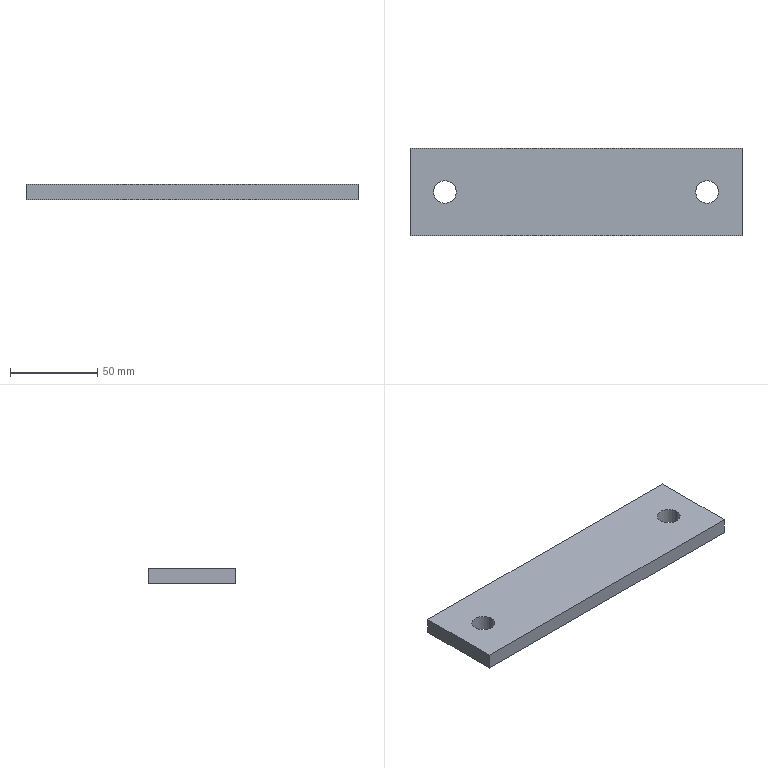Part | STEP file | DCV-000-026 | 1 solid | 10 faces | box 190 x 50 x 9 mm | volume 83111 mm3 | plane 6 | cylinder 4 | commonest cylinder face diameters 13 x4
STEP:
#1=CARTESIAN_POINT('',(0.,0.,0.));
#2=DIRECTION('',(0.,0.,1.));
#3=DIRECTION('',(1.,0.,0.));
#4=AXIS2_PLACEMENT_3D('',#1,#2,#3);
#5=CARTESIAN_POINT('',(81.5,0.,0.));
#6=VERTEX_POINT('',#5);
#7=CARTESIAN_POINT('',(81.5,0.,9.));
#8=VERTEX_POINT('',#7);
#9=CARTESIAN_POINT('',(81.5,0.,-187.675));
#10=DIRECTION('',(0.,0.,1.));
#11=VECTOR('',#10,1.);
#12=LINE('',#9,#11);
#13=CARTESIAN_POINT('',(75.,0.,-187.675));
#14=DIRECTION('',(0.,0.,1.));
#15=DIRECTION('',(1.,0.,0.));
#16=AXIS2_PLACEMENT_3D('',#13,#14,#15);
#17=CYLINDRICAL_SURFACE('',#16,6.5);
#18=CARTESIAN_POINT('',(6.283,0.));
#19=DIRECTION('',(0.,1.));
#20=VECTOR('',#19,1.);
#21=LINE('',#18,#20);
#22=(GEOMETRIC_REPRESENTATION_CONTEXT(2)PARAMETRIC_REPRESENTATION_CONTEXT()REPRESENTATION_CONTEXT('',''));
#23=DEFINITIONAL_REPRESENTATION('',(#21),#22);
#24=PCURVE('',#17,#23);
#25=CARTESIAN_POINT('',(75.,0.,-187.675));
#26=DIRECTION('',(0.,0.,1.));
#27=DIRECTION('',(1.,0.,0.));
#28=AXIS2_PLACEMENT_3D('',#25,#26,#27);
#29=CYLINDRICAL_SURFACE('',#28,6.5);
#30=CARTESIAN_POINT('',(0.,0.));
#31=DIRECTION('',(0.,1.));
#32=VECTOR('',#31,1.);
#33=LINE('',#30,#32);
#34=(GEOMETRIC_REPRESENTATION_CONTEXT(2)PARAMETRIC_REPRESENTATION_CONTEXT()REPRESENTATION_CONTEXT('',''));
#35=DEFINITIONAL_REPRESENTATION('',(#33),#34);
#36=PCURVE('',#29,#35);
#37=SURFACE_CURVE('',#12,(#24,#36),.PCURVE_S1.);
#38=EDGE_CURVE('',#6,#8,#37,.T.);
#39=ORIENTED_EDGE('',*,*,#38,.T.);
#40=CARTESIAN_POINT('',(68.5,0.,9.));
#41=VERTEX_POINT('',#40);
#42=CARTESIAN_POINT('',(75.,0.,9.));
#43=DIRECTION('',(0.,0.,-1.));
#44=DIRECTION('',(1.,0.,0.));
#45=AXIS2_PLACEMENT_3D('',#42,#43,#44);
#46=CIRCLE('',#45,6.5);
#47=CARTESIAN_POINT('',(6.283,196.675));
#48=DIRECTION('',(-1.,0.));
#49=VECTOR('',#48,1.);
#50=LINE('',#47,#49);
#51=(GEOMETRIC_REPRESENTATION_CONTEXT(2)PARAMETRIC_REPRESENTATION_CONTEXT()REPRESENTATION_CONTEXT('',''));
#52=DEFINITIONAL_REPRESENTATION('',(#50),#51);
#53=PCURVE('',#17,#52);
#54=CARTESIAN_POINT('',(0.,0.,9.));
#55=DIRECTION('',(0.,0.,1.));
#56=DIRECTION('',(1.,0.,0.));
#57=AXIS2_PLACEMENT_3D('',#54,#55,#56);
#58=PLANE('',#57);
#59=CARTESIAN_POINT('',(81.5,0.));
#60=CARTESIAN_POINT('',(81.5,-11.258));
#61=CARTESIAN_POINT('',(71.75,-5.629));
#62=CARTESIAN_POINT('',(62.,0.));
#63=CARTESIAN_POINT('',(71.75,5.629));
#64=CARTESIAN_POINT('',(81.5,11.258));
#65=CARTESIAN_POINT('',(81.5,0.));
#66=(BOUNDED_CURVE()B_SPLINE_CURVE(2,(#59,#60,#61,#62,#63,#64,#65),.UNSPECIFIED.,.T.,.F.)B_SPLINE_CURVE_WITH_KNOTS((1,2,2,2,2,1),(-2.094,0.,2.094,4.189,6.283,8.378),.UNSPECIFIED.)CURVE()GEOMETRIC_REPRESENTATION_ITEM()RATIONAL_B_SPLINE_CURVE((1.,0.5,1.,0.5,1.,0.5,1.))REPRESENTATION_ITEM(''));
#67=(GEOMETRIC_REPRESENTATION_CONTEXT(2)PARAMETRIC_REPRESENTATION_CONTEXT()REPRESENTATION_CONTEXT('',''));
#68=DEFINITIONAL_REPRESENTATION('',(#66),#67);
#69=PCURVE('',#58,#68);
#70=SURFACE_CURVE('',#46,(#53,#69),.PCURVE_S1.);
#71=EDGE_CURVE('',#8,#41,#70,.T.);
#72=ORIENTED_EDGE('',*,*,#71,.T.);
#73=CARTESIAN_POINT('',(68.5,0.,0.));
#74=VERTEX_POINT('',#73);
#75=CARTESIAN_POINT('',(68.5,0.,-187.675));
#76=DIRECTION('',(0.,0.,1.));
#77=VECTOR('',#76,1.);
#78=LINE('',#75,#77);
#79=CARTESIAN_POINT('',(3.142,0.));
#80=DIRECTION('',(0.,1.));
#81=VECTOR('',#80,1.);
#82=LINE('',#79,#81);
#83=(GEOMETRIC_REPRESENTATION_CONTEXT(2)PARAMETRIC_REPRESENTATION_CONTEXT()REPRESENTATION_CONTEXT('',''));
#84=DEFINITIONAL_REPRESENTATION('',(#82),#83);
#85=PCURVE('',#17,#84);
#86=CARTESIAN_POINT('',(3.142,0.));
#87=DIRECTION('',(0.,1.));
#88=VECTOR('',#87,1.);
#89=LINE('',#86,#88);
#90=(GEOMETRIC_REPRESENTATION_CONTEXT(2)PARAMETRIC_REPRESENTATION_CONTEXT()REPRESENTATION_CONTEXT('',''));
#91=DEFINITIONAL_REPRESENTATION('',(#89),#90);
#92=PCURVE('',#29,#91);
#93=SURFACE_CURVE('',#78,(#85,#92),.PCURVE_S1.);
#94=EDGE_CURVE('',#74,#41,#93,.T.);
#95=ORIENTED_EDGE('',*,*,#94,.F.);
#96=CARTESIAN_POINT('',(75.,0.,0.));
#97=DIRECTION('',(0.,0.,1.));
#98=DIRECTION('',(1.,0.,0.));
#99=AXIS2_PLACEMENT_3D('',#96,#97,#98);
#100=CIRCLE('',#99,6.5);
#101=CARTESIAN_POINT('',(0.,187.675));
#102=DIRECTION('',(1.,0.));
#103=VECTOR('',#102,1.);
#104=LINE('',#101,#103);
#105=(GEOMETRIC_REPRESENTATION_CONTEXT(2)PARAMETRIC_REPRESENTATION_CONTEXT()REPRESENTATION_CONTEXT('',''));
#106=DEFINITIONAL_REPRESENTATION('',(#104),#105);
#107=PCURVE('',#17,#106);
#108=CARTESIAN_POINT('',(0.,0.,0.));
#109=DIRECTION('',(0.,0.,1.));
#110=DIRECTION('',(1.,0.,0.));
#111=AXIS2_PLACEMENT_3D('',#108,#109,#110);
#112=PLANE('',#111);
#113=CARTESIAN_POINT('',(75.,0.));
#114=DIRECTION('',(1.,0.));
#115=AXIS2_PLACEMENT_2D('',#113,#114);
#116=CIRCLE('',#115,6.5);
#117=(GEOMETRIC_REPRESENTATION_CONTEXT(2)PARAMETRIC_REPRESENTATION_CONTEXT()REPRESENTATION_CONTEXT('',''));
#118=DEFINITIONAL_REPRESENTATION('',(#116),#117);
#119=PCURVE('',#112,#118);
#120=SURFACE_CURVE('',#100,(#107,#119),.PCURVE_S1.);
#121=EDGE_CURVE('',#74,#6,#120,.T.);
#122=ORIENTED_EDGE('',*,*,#121,.T.);
#123=EDGE_LOOP('',(#39,#72,#95,#122));
#124=FACE_BOUND('',#123,.F.);
#125=ADVANCED_FACE('',(#124),#17,.F.);
#126=CARTESIAN_POINT('',(-68.5,0.,0.));
#127=VERTEX_POINT('',#126);
#128=CARTESIAN_POINT('',(-68.5,0.,9.));
#129=VERTEX_POINT('',#128);
#130=CARTESIAN_POINT('',(-68.5,0.,-187.675));
#131=DIRECTION('',(0.,0.,1.));
#132=VECTOR('',#131,1.);
#133=LINE('',#130,#132);
#134=CARTESIAN_POINT('',(-75.,0.,-187.675));
#135=DIRECTION('',(0.,0.,1.));
#136=DIRECTION('',(1.,0.,0.));
#137=AXIS2_PLACEMENT_3D('',#134,#135,#136);
#138=CYLINDRICAL_SURFACE('',#137,6.5);
#139=CARTESIAN_POINT('',(6.283,0.));
#140=DIRECTION('',(0.,1.));
#141=VECTOR('',#140,1.);
#142=LINE('',#139,#141);
#143=(GEOMETRIC_REPRESENTATION_CONTEXT(2)PARAMETRIC_REPRESENTATION_CONTEXT()REPRESENTATION_CONTEXT('',''));
#144=DEFINITIONAL_REPRESENTATION('',(#142),#143);
#145=PCURVE('',#138,#144);
#146=CARTESIAN_POINT('',(-75.,0.,-187.675));
#147=DIRECTION('',(0.,0.,1.));
#148=DIRECTION('',(1.,0.,0.));
#149=AXIS2_PLACEMENT_3D('',#146,#147,#148);
#150=CYLINDRICAL_SURFACE('',#149,6.5);
#151=CARTESIAN_POINT('',(0.,0.));
#152=DIRECTION('',(0.,1.));
#153=VECTOR('',#152,1.);
#154=LINE('',#151,#153);
#155=(GEOMETRIC_REPRESENTATION_CONTEXT(2)PARAMETRIC_REPRESENTATION_CONTEXT()REPRESENTATION_CONTEXT('',''));
#156=DEFINITIONAL_REPRESENTATION('',(#154),#155);
#157=PCURVE('',#150,#156);
#158=SURFACE_CURVE('',#133,(#145,#157),.PCURVE_S1.);
#159=EDGE_CURVE('',#127,#129,#158,.T.);
#160=ORIENTED_EDGE('',*,*,#159,.T.);
#161=CARTESIAN_POINT('',(-81.5,0.,9.));
#162=VERTEX_POINT('',#161);
#163=CARTESIAN_POINT('',(-75.,0.,9.));
#164=DIRECTION('',(0.,0.,-1.));
#165=DIRECTION('',(1.,0.,0.));
#166=AXIS2_PLACEMENT_3D('',#163,#164,#165);
#167=CIRCLE('',#166,6.5);
#168=CARTESIAN_POINT('',(6.283,196.675));
#169=DIRECTION('',(-1.,0.));
#170=VECTOR('',#169,1.);
#171=LINE('',#168,#170);
#172=(GEOMETRIC_REPRESENTATION_CONTEXT(2)PARAMETRIC_REPRESENTATION_CONTEXT()REPRESENTATION_CONTEXT('',''));
#173=DEFINITIONAL_REPRESENTATION('',(#171),#172);
#174=PCURVE('',#138,#173);
#175=CARTESIAN_POINT('',(-68.5,0.));
#176=CARTESIAN_POINT('',(-68.5,-11.258));
#177=CARTESIAN_POINT('',(-78.25,-5.629));
#178=CARTESIAN_POINT('',(-88.,0.));
#179=CARTESIAN_POINT('',(-78.25,5.629));
#180=CARTESIAN_POINT('',(-68.5,11.258));
#181=CARTESIAN_POINT('',(-68.5,0.));
#182=(BOUNDED_CURVE()B_SPLINE_CURVE(2,(#175,#176,#177,#178,#179,#180,#181),.UNSPECIFIED.,.T.,.F.)B_SPLINE_CURVE_WITH_KNOTS((1,2,2,2,2,1),(-2.094,0.,2.094,4.189,6.283,8.378),.UNSPECIFIED.)CURVE()GEOMETRIC_REPRESENTATION_ITEM()RATIONAL_B_SPLINE_CURVE((1.,0.5,1.,0.5,1.,0.5,1.))REPRESENTATION_ITEM(''));
#183=(GEOMETRIC_REPRESENTATION_CONTEXT(2)PARAMETRIC_REPRESENTATION_CONTEXT()REPRESENTATION_CONTEXT('',''));
#184=DEFINITIONAL_REPRESENTATION('',(#182),#183);
#185=PCURVE('',#58,#184);
#186=SURFACE_CURVE('',#167,(#174,#185),.PCURVE_S1.);
#187=EDGE_CURVE('',#129,#162,#186,.T.);
#188=ORIENTED_EDGE('',*,*,#187,.T.);
#189=CARTESIAN_POINT('',(-81.5,0.,0.));
#190=VERTEX_POINT('',#189);
#191=CARTESIAN_POINT('',(-81.5,0.,-187.675));
#192=DIRECTION('',(0.,0.,1.));
#193=VECTOR('',#192,1.);
#194=LINE('',#191,#193);
#195=CARTESIAN_POINT('',(3.142,0.));
#196=DIRECTION('',(0.,1.));
#197=VECTOR('',#196,1.);
#198=LINE('',#195,#197);
#199=(GEOMETRIC_REPRESENTATION_CONTEXT(2)PARAMETRIC_REPRESENTATION_CONTEXT()REPRESENTATION_CONTEXT('',''));
#200=DEFINITIONAL_REPRESENTATION('',(#198),#199);
#201=PCURVE('',#138,#200);
#202=CARTESIAN_POINT('',(3.142,0.));
#203=DIRECTION('',(0.,1.));
#204=VECTOR('',#203,1.);
#205=LINE('',#202,#204);
#206=(GEOMETRIC_REPRESENTATION_CONTEXT(2)PARAMETRIC_REPRESENTATION_CONTEXT()REPRESENTATION_CONTEXT('',''));
#207=DEFINITIONAL_REPRESENTATION('',(#205),#206);
#208=PCURVE('',#150,#207);
#209=SURFACE_CURVE('',#194,(#201,#208),.PCURVE_S1.);
#210=EDGE_CURVE('',#190,#162,#209,.T.);
#211=ORIENTED_EDGE('',*,*,#210,.F.);
#212=CARTESIAN_POINT('',(-75.,0.,0.));
#213=DIRECTION('',(0.,0.,1.));
#214=DIRECTION('',(1.,0.,0.));
#215=AXIS2_PLACEMENT_3D('',#212,#213,#214);
#216=CIRCLE('',#215,6.5);
#217=CARTESIAN_POINT('',(0.,187.675));
#218=DIRECTION('',(1.,0.));
#219=VECTOR('',#218,1.);
#220=LINE('',#217,#219);
#221=(GEOMETRIC_REPRESENTATION_CONTEXT(2)PARAMETRIC_REPRESENTATION_CONTEXT()REPRESENTATION_CONTEXT('',''));
#222=DEFINITIONAL_REPRESENTATION('',(#220),#221);
#223=PCURVE('',#138,#222);
#224=CARTESIAN_POINT('',(-75.,0.));
#225=DIRECTION('',(1.,0.));
#226=AXIS2_PLACEMENT_2D('',#224,#225);
#227=CIRCLE('',#226,6.5);
#228=(GEOMETRIC_REPRESENTATION_CONTEXT(2)PARAMETRIC_REPRESENTATION_CONTEXT()REPRESENTATION_CONTEXT('',''));
#229=DEFINITIONAL_REPRESENTATION('',(#227),#228);
#230=PCURVE('',#112,#229);
#231=SURFACE_CURVE('',#216,(#223,#230),.PCURVE_S1.);
#232=EDGE_CURVE('',#190,#127,#231,.T.);
#233=ORIENTED_EDGE('',*,*,#232,.T.);
#234=EDGE_LOOP('',(#160,#188,#211,#233));
#235=FACE_BOUND('',#234,.F.);
#236=ADVANCED_FACE('',(#235),#138,.F.);
#237=CARTESIAN_POINT('',(-75.,0.,0.));
#238=DIRECTION('',(0.,0.,1.));
#239=DIRECTION('',(1.,0.,0.));
#240=AXIS2_PLACEMENT_3D('',#237,#238,#239);
#241=CIRCLE('',#240,6.5);
#242=CARTESIAN_POINT('',(-75.,0.));
#243=DIRECTION('',(1.,0.));
#244=AXIS2_PLACEMENT_2D('',#242,#243);
#245=CIRCLE('',#244,6.5);
#246=(GEOMETRIC_REPRESENTATION_CONTEXT(2)PARAMETRIC_REPRESENTATION_CONTEXT()REPRESENTATION_CONTEXT('',''));
#247=DEFINITIONAL_REPRESENTATION('',(#245),#246);
#248=PCURVE('',#112,#247);
#249=CARTESIAN_POINT('',(0.,187.675));
#250=DIRECTION('',(1.,0.));
#251=VECTOR('',#250,1.);
#252=LINE('',#249,#251);
#253=(GEOMETRIC_REPRESENTATION_CONTEXT(2)PARAMETRIC_REPRESENTATION_CONTEXT()REPRESENTATION_CONTEXT('',''));
#254=DEFINITIONAL_REPRESENTATION('',(#252),#253);
#255=PCURVE('',#150,#254);
#256=SURFACE_CURVE('',#241,(#248,#255),.PCURVE_S1.);
#257=EDGE_CURVE('',#127,#190,#256,.T.);
#258=ORIENTED_EDGE('',*,*,#257,.T.);
#259=ORIENTED_EDGE('',*,*,#232,.T.);
#260=EDGE_LOOP('',(#258,#259));
#261=FACE_BOUND('',#260,.T.);
#262=CARTESIAN_POINT('',(75.,0.,0.));
#263=DIRECTION('',(0.,0.,1.));
#264=DIRECTION('',(1.,0.,0.));
#265=AXIS2_PLACEMENT_3D('',#262,#263,#264);
#266=CIRCLE('',#265,6.5);
#267=CARTESIAN_POINT('',(75.,0.));
#268=DIRECTION('',(1.,0.));
#269=AXIS2_PLACEMENT_2D('',#267,#268);
#270=CIRCLE('',#269,6.5);
#271=(GEOMETRIC_REPRESENTATION_CONTEXT(2)PARAMETRIC_REPRESENTATION_CONTEXT()REPRESENTATION_CONTEXT('',''));
#272=DEFINITIONAL_REPRESENTATION('',(#270),#271);
#273=PCURVE('',#112,#272);
#274=CARTESIAN_POINT('',(0.,187.675));
#275=DIRECTION('',(1.,0.));
#276=VECTOR('',#275,1.);
#277=LINE('',#274,#276);
#278=(GEOMETRIC_REPRESENTATION_CONTEXT(2)PARAMETRIC_REPRESENTATION_CONTEXT()REPRESENTATION_CONTEXT('',''));
#279=DEFINITIONAL_REPRESENTATION('',(#277),#278);
#280=PCURVE('',#29,#279);
#281=SURFACE_CURVE('',#266,(#273,#280),.PCURVE_S1.);
#282=EDGE_CURVE('',#6,#74,#281,.T.);
#283=ORIENTED_EDGE('',*,*,#282,.T.);
#284=ORIENTED_EDGE('',*,*,#121,.T.);
#285=EDGE_LOOP('',(#283,#284));
#286=FACE_BOUND('',#285,.T.);
#287=CARTESIAN_POINT('',(95.,-25.,0.));
#288=VERTEX_POINT('',#287);
#289=CARTESIAN_POINT('',(95.,25.,0.));
#290=VERTEX_POINT('',#289);
#291=CARTESIAN_POINT('',(95.,-25.,0.));
#292=DIRECTION('',(0.,1.,0.));
#293=VECTOR('',#292,1.);
#294=LINE('',#291,#293);
#295=CARTESIAN_POINT('',(95.,-25.));
#296=DIRECTION('',(0.,1.));
#297=VECTOR('',#296,1.);
#298=LINE('',#295,#297);
#299=(GEOMETRIC_REPRESENTATION_CONTEXT(2)PARAMETRIC_REPRESENTATION_CONTEXT()REPRESENTATION_CONTEXT('',''));
#300=DEFINITIONAL_REPRESENTATION('',(#298),#299);
#301=PCURVE('',#112,#300);
#302=CARTESIAN_POINT('',(95.,-25.,0.));
#303=DIRECTION('',(1.,0.,0.));
#304=DIRECTION('',(0.,1.,0.));
#305=AXIS2_PLACEMENT_3D('',#302,#303,#304);
#306=PLANE('',#305);
#307=CARTESIAN_POINT('',(0.,0.));
#308=DIRECTION('',(1.,0.));
#309=VECTOR('',#308,1.);
#310=LINE('',#307,#309);
#311=(GEOMETRIC_REPRESENTATION_CONTEXT(2)PARAMETRIC_REPRESENTATION_CONTEXT()REPRESENTATION_CONTEXT('',''));
#312=DEFINITIONAL_REPRESENTATION('',(#310),#311);
#313=PCURVE('',#306,#312);
#314=SURFACE_CURVE('',#294,(#301,#313),.PCURVE_S1.);
#315=EDGE_CURVE('',#288,#290,#314,.T.);
#316=ORIENTED_EDGE('',*,*,#315,.F.);
#317=CARTESIAN_POINT('',(-95.,-25.,0.));
#318=VERTEX_POINT('',#317);
#319=CARTESIAN_POINT('',(-95.,-25.,0.));
#320=DIRECTION('',(1.,0.,0.));
#321=VECTOR('',#320,1.);
#322=LINE('',#319,#321);
#323=CARTESIAN_POINT('',(-95.,-25.));
#324=DIRECTION('',(1.,0.));
#325=VECTOR('',#324,1.);
#326=LINE('',#323,#325);
#327=(GEOMETRIC_REPRESENTATION_CONTEXT(2)PARAMETRIC_REPRESENTATION_CONTEXT()REPRESENTATION_CONTEXT('',''));
#328=DEFINITIONAL_REPRESENTATION('',(#326),#327);
#329=PCURVE('',#112,#328);
#330=CARTESIAN_POINT('',(-95.,-25.,0.));
#331=DIRECTION('',(0.,-1.,0.));
#332=DIRECTION('',(0.,0.,-1.));
#333=AXIS2_PLACEMENT_3D('',#330,#331,#332);
#334=PLANE('',#333);
#335=CARTESIAN_POINT('',(0.,0.));
#336=DIRECTION('',(0.,1.));
#337=VECTOR('',#336,1.);
#338=LINE('',#335,#337);
#339=(GEOMETRIC_REPRESENTATION_CONTEXT(2)PARAMETRIC_REPRESENTATION_CONTEXT()REPRESENTATION_CONTEXT('',''));
#340=DEFINITIONAL_REPRESENTATION('',(#338),#339);
#341=PCURVE('',#334,#340);
#342=SURFACE_CURVE('',#322,(#329,#341),.PCURVE_S1.);
#343=EDGE_CURVE('',#318,#288,#342,.T.);
#344=ORIENTED_EDGE('',*,*,#343,.F.);
#345=CARTESIAN_POINT('',(-95.,25.,0.));
#346=VERTEX_POINT('',#345);
#347=CARTESIAN_POINT('',(-95.,25.,0.));
#348=DIRECTION('',(0.,-1.,0.));
#349=VECTOR('',#348,1.);
#350=LINE('',#347,#349);
#351=CARTESIAN_POINT('',(-95.,25.));
#352=DIRECTION('',(0.,-1.));
#353=VECTOR('',#352,1.);
#354=LINE('',#351,#353);
#355=(GEOMETRIC_REPRESENTATION_CONTEXT(2)PARAMETRIC_REPRESENTATION_CONTEXT()REPRESENTATION_CONTEXT('',''));
#356=DEFINITIONAL_REPRESENTATION('',(#354),#355);
#357=PCURVE('',#112,#356);
#358=CARTESIAN_POINT('',(-95.,25.,0.));
#359=DIRECTION('',(-1.,0.,0.));
#360=DIRECTION('',(0.,0.,1.));
#361=AXIS2_PLACEMENT_3D('',#358,#359,#360);
#362=PLANE('',#361);
#363=CARTESIAN_POINT('',(0.,0.));
#364=DIRECTION('',(0.,-1.));
#365=VECTOR('',#364,1.);
#366=LINE('',#363,#365);
#367=(GEOMETRIC_REPRESENTATION_CONTEXT(2)PARAMETRIC_REPRESENTATION_CONTEXT()REPRESENTATION_CONTEXT('',''));
#368=DEFINITIONAL_REPRESENTATION('',(#366),#367);
#369=PCURVE('',#362,#368);
#370=SURFACE_CURVE('',#350,(#357,#369),.PCURVE_S1.);
#371=EDGE_CURVE('',#346,#318,#370,.T.);
#372=ORIENTED_EDGE('',*,*,#371,.F.);
#373=CARTESIAN_POINT('',(95.,25.,0.));
#374=DIRECTION('',(-1.,0.,0.));
#375=VECTOR('',#374,1.);
#376=LINE('',#373,#375);
#377=CARTESIAN_POINT('',(95.,25.));
#378=DIRECTION('',(-1.,0.));
#379=VECTOR('',#378,1.);
#380=LINE('',#377,#379);
#381=(GEOMETRIC_REPRESENTATION_CONTEXT(2)PARAMETRIC_REPRESENTATION_CONTEXT()REPRESENTATION_CONTEXT('',''));
#382=DEFINITIONAL_REPRESENTATION('',(#380),#381);
#383=PCURVE('',#112,#382);
#384=CARTESIAN_POINT('',(95.,25.,0.));
#385=DIRECTION('',(0.,1.,0.));
#386=DIRECTION('',(1.,0.,0.));
#387=AXIS2_PLACEMENT_3D('',#384,#385,#386);
#388=PLANE('',#387);
#389=CARTESIAN_POINT('',(0.,0.));
#390=DIRECTION('',(-1.,0.));
#391=VECTOR('',#390,1.);
#392=LINE('',#389,#391);
#393=(GEOMETRIC_REPRESENTATION_CONTEXT(2)PARAMETRIC_REPRESENTATION_CONTEXT()REPRESENTATION_CONTEXT('',''));
#394=DEFINITIONAL_REPRESENTATION('',(#392),#393);
#395=PCURVE('',#388,#394);
#396=SURFACE_CURVE('',#376,(#383,#395),.PCURVE_S1.);
#397=EDGE_CURVE('',#290,#346,#396,.T.);
#398=ORIENTED_EDGE('',*,*,#397,.F.);
#399=EDGE_LOOP('',(#316,#344,#372,#398));
#400=FACE_BOUND('',#399,.T.);
#401=ADVANCED_FACE('',(#261,#286,#400),#112,.F.);
#402=ORIENTED_EDGE('',*,*,#187,.T.);
#403=CARTESIAN_POINT('',(-75.,0.,9.));
#404=DIRECTION('',(0.,0.,-1.));
#405=DIRECTION('',(1.,0.,0.));
#406=AXIS2_PLACEMENT_3D('',#403,#404,#405);
#407=CIRCLE('',#406,6.5);
#408=CARTESIAN_POINT('',(-68.5,0.));
#409=CARTESIAN_POINT('',(-68.5,-11.258));
#410=CARTESIAN_POINT('',(-78.25,-5.629));
#411=CARTESIAN_POINT('',(-88.,0.));
#412=CARTESIAN_POINT('',(-78.25,5.629));
#413=CARTESIAN_POINT('',(-68.5,11.258));
#414=CARTESIAN_POINT('',(-68.5,0.));
#415=(BOUNDED_CURVE()B_SPLINE_CURVE(2,(#408,#409,#410,#411,#412,#413,#414),.UNSPECIFIED.,.T.,.F.)B_SPLINE_CURVE_WITH_KNOTS((1,2,2,2,2,1),(-2.094,0.,2.094,4.189,6.283,8.378),.UNSPECIFIED.)CURVE()GEOMETRIC_REPRESENTATION_ITEM()RATIONAL_B_SPLINE_CURVE((1.,0.5,1.,0.5,1.,0.5,1.))REPRESENTATION_ITEM(''));
#416=(GEOMETRIC_REPRESENTATION_CONTEXT(2)PARAMETRIC_REPRESENTATION_CONTEXT()REPRESENTATION_CONTEXT('',''));
#417=DEFINITIONAL_REPRESENTATION('',(#415),#416);
#418=PCURVE('',#58,#417);
#419=CARTESIAN_POINT('',(6.283,196.675));
#420=DIRECTION('',(-1.,0.));
#421=VECTOR('',#420,1.);
#422=LINE('',#419,#421);
#423=(GEOMETRIC_REPRESENTATION_CONTEXT(2)PARAMETRIC_REPRESENTATION_CONTEXT()REPRESENTATION_CONTEXT('',''));
#424=DEFINITIONAL_REPRESENTATION('',(#422),#423);
#425=PCURVE('',#150,#424);
#426=SURFACE_CURVE('',#407,(#418,#425),.PCURVE_S1.);
#427=EDGE_CURVE('',#162,#129,#426,.T.);
#428=ORIENTED_EDGE('',*,*,#427,.T.);
#429=EDGE_LOOP('',(#402,#428));
#430=FACE_BOUND('',#429,.T.);
#431=ORIENTED_EDGE('',*,*,#71,.T.);
#432=CARTESIAN_POINT('',(75.,0.,9.));
#433=DIRECTION('',(0.,0.,-1.));
#434=DIRECTION('',(1.,0.,0.));
#435=AXIS2_PLACEMENT_3D('',#432,#433,#434);
#436=CIRCLE('',#435,6.5);
#437=CARTESIAN_POINT('',(81.5,0.));
#438=CARTESIAN_POINT('',(81.5,-11.258));
#439=CARTESIAN_POINT('',(71.75,-5.629));
#440=CARTESIAN_POINT('',(62.,0.));
#441=CARTESIAN_POINT('',(71.75,5.629));
#442=CARTESIAN_POINT('',(81.5,11.258));
#443=CARTESIAN_POINT('',(81.5,0.));
#444=(BOUNDED_CURVE()B_SPLINE_CURVE(2,(#437,#438,#439,#440,#441,#442,#443),.UNSPECIFIED.,.T.,.F.)B_SPLINE_CURVE_WITH_KNOTS((1,2,2,2,2,1),(-2.094,0.,2.094,4.189,6.283,8.378),.UNSPECIFIED.)CURVE()GEOMETRIC_REPRESENTATION_ITEM()RATIONAL_B_SPLINE_CURVE((1.,0.5,1.,0.5,1.,0.5,1.))REPRESENTATION_ITEM(''));
#445=(GEOMETRIC_REPRESENTATION_CONTEXT(2)PARAMETRIC_REPRESENTATION_CONTEXT()REPRESENTATION_CONTEXT('',''));
#446=DEFINITIONAL_REPRESENTATION('',(#444),#445);
#447=PCURVE('',#58,#446);
#448=CARTESIAN_POINT('',(6.283,196.675));
#449=DIRECTION('',(-1.,0.));
#450=VECTOR('',#449,1.);
#451=LINE('',#448,#450);
#452=(GEOMETRIC_REPRESENTATION_CONTEXT(2)PARAMETRIC_REPRESENTATION_CONTEXT()REPRESENTATION_CONTEXT('',''));
#453=DEFINITIONAL_REPRESENTATION('',(#451),#452);
#454=PCURVE('',#29,#453);
#455=SURFACE_CURVE('',#436,(#447,#454),.PCURVE_S1.);
#456=EDGE_CURVE('',#41,#8,#455,.T.);
#457=ORIENTED_EDGE('',*,*,#456,.T.);
#458=EDGE_LOOP('',(#431,#457));
#459=FACE_BOUND('',#458,.T.);
#460=CARTESIAN_POINT('',(95.,-25.,9.));
#461=VERTEX_POINT('',#460);
#462=CARTESIAN_POINT('',(95.,25.,9.));
#463=VERTEX_POINT('',#462);
#464=CARTESIAN_POINT('',(95.,-25.,9.));
#465=DIRECTION('',(0.,1.,0.));
#466=VECTOR('',#465,1.);
#467=LINE('',#464,#466);
#468=CARTESIAN_POINT('',(95.,-25.));
#469=DIRECTION('',(0.,1.));
#470=VECTOR('',#469,1.);
#471=LINE('',#468,#470);
#472=(GEOMETRIC_REPRESENTATION_CONTEXT(2)PARAMETRIC_REPRESENTATION_CONTEXT()REPRESENTATION_CONTEXT('',''));
#473=DEFINITIONAL_REPRESENTATION('',(#471),#472);
#474=PCURVE('',#58,#473);
#475=CARTESIAN_POINT('',(0.,9.));
#476=DIRECTION('',(1.,0.));
#477=VECTOR('',#476,1.);
#478=LINE('',#475,#477);
#479=(GEOMETRIC_REPRESENTATION_CONTEXT(2)PARAMETRIC_REPRESENTATION_CONTEXT()REPRESENTATION_CONTEXT('',''));
#480=DEFINITIONAL_REPRESENTATION('',(#478),#479);
#481=PCURVE('',#306,#480);
#482=SURFACE_CURVE('',#467,(#474,#481),.PCURVE_S1.);
#483=EDGE_CURVE('',#461,#463,#482,.T.);
#484=ORIENTED_EDGE('',*,*,#483,.T.);
#485=CARTESIAN_POINT('',(-95.,25.,9.));
#486=VERTEX_POINT('',#485);
#487=CARTESIAN_POINT('',(95.,25.,9.));
#488=DIRECTION('',(-1.,0.,0.));
#489=VECTOR('',#488,1.);
#490=LINE('',#487,#489);
#491=CARTESIAN_POINT('',(95.,25.));
#492=DIRECTION('',(-1.,0.));
#493=VECTOR('',#492,1.);
#494=LINE('',#491,#493);
#495=(GEOMETRIC_REPRESENTATION_CONTEXT(2)PARAMETRIC_REPRESENTATION_CONTEXT()REPRESENTATION_CONTEXT('',''));
#496=DEFINITIONAL_REPRESENTATION('',(#494),#495);
#497=PCURVE('',#58,#496);
#498=CARTESIAN_POINT('',(0.,-9.));
#499=DIRECTION('',(-1.,0.));
#500=VECTOR('',#499,1.);
#501=LINE('',#498,#500);
#502=(GEOMETRIC_REPRESENTATION_CONTEXT(2)PARAMETRIC_REPRESENTATION_CONTEXT()REPRESENTATION_CONTEXT('',''));
#503=DEFINITIONAL_REPRESENTATION('',(#501),#502);
#504=PCURVE('',#388,#503);
#505=SURFACE_CURVE('',#490,(#497,#504),.PCURVE_S1.);
#506=EDGE_CURVE('',#463,#486,#505,.T.);
#507=ORIENTED_EDGE('',*,*,#506,.T.);
#508=CARTESIAN_POINT('',(-95.,-25.,9.));
#509=VERTEX_POINT('',#508);
#510=CARTESIAN_POINT('',(-95.,25.,9.));
#511=DIRECTION('',(0.,-1.,0.));
#512=VECTOR('',#511,1.);
#513=LINE('',#510,#512);
#514=CARTESIAN_POINT('',(-95.,25.));
#515=DIRECTION('',(0.,-1.));
#516=VECTOR('',#515,1.);
#517=LINE('',#514,#516);
#518=(GEOMETRIC_REPRESENTATION_CONTEXT(2)PARAMETRIC_REPRESENTATION_CONTEXT()REPRESENTATION_CONTEXT('',''));
#519=DEFINITIONAL_REPRESENTATION('',(#517),#518);
#520=PCURVE('',#58,#519);
#521=CARTESIAN_POINT('',(9.,0.));
#522=DIRECTION('',(0.,-1.));
#523=VECTOR('',#522,1.);
#524=LINE('',#521,#523);
#525=(GEOMETRIC_REPRESENTATION_CONTEXT(2)PARAMETRIC_REPRESENTATION_CONTEXT()REPRESENTATION_CONTEXT('',''));
#526=DEFINITIONAL_REPRESENTATION('',(#524),#525);
#527=PCURVE('',#362,#526);
#528=SURFACE_CURVE('',#513,(#520,#527),.PCURVE_S1.);
#529=EDGE_CURVE('',#486,#509,#528,.T.);
#530=ORIENTED_EDGE('',*,*,#529,.T.);
#531=CARTESIAN_POINT('',(-95.,-25.,9.));
#532=DIRECTION('',(1.,0.,0.));
#533=VECTOR('',#532,1.);
#534=LINE('',#531,#533);
#535=CARTESIAN_POINT('',(-95.,-25.));
#536=DIRECTION('',(1.,0.));
#537=VECTOR('',#536,1.);
#538=LINE('',#535,#537);
#539=(GEOMETRIC_REPRESENTATION_CONTEXT(2)PARAMETRIC_REPRESENTATION_CONTEXT()REPRESENTATION_CONTEXT('',''));
#540=DEFINITIONAL_REPRESENTATION('',(#538),#539);
#541=PCURVE('',#58,#540);
#542=CARTESIAN_POINT('',(-9.,0.));
#543=DIRECTION('',(0.,1.));
#544=VECTOR('',#543,1.);
#545=LINE('',#542,#544);
#546=(GEOMETRIC_REPRESENTATION_CONTEXT(2)PARAMETRIC_REPRESENTATION_CONTEXT()REPRESENTATION_CONTEXT('',''));
#547=DEFINITIONAL_REPRESENTATION('',(#545),#546);
#548=PCURVE('',#334,#547);
#549=SURFACE_CURVE('',#534,(#541,#548),.PCURVE_S1.);
#550=EDGE_CURVE('',#509,#461,#549,.T.);
#551=ORIENTED_EDGE('',*,*,#550,.T.);
#552=EDGE_LOOP('',(#484,#507,#530,#551));
#553=FACE_BOUND('',#552,.T.);
#554=ADVANCED_FACE('',(#430,#459,#553),#58,.T.);
#555=ORIENTED_EDGE('',*,*,#315,.T.);
#556=CARTESIAN_POINT('',(95.,25.,0.));
#557=DIRECTION('',(0.,0.,1.));
#558=VECTOR('',#557,1.);
#559=LINE('',#556,#558);
#560=CARTESIAN_POINT('',(50.,0.));
#561=DIRECTION('',(0.,1.));
#562=VECTOR('',#561,1.);
#563=LINE('',#560,#562);
#564=(GEOMETRIC_REPRESENTATION_CONTEXT(2)PARAMETRIC_REPRESENTATION_CONTEXT()REPRESENTATION_CONTEXT('',''));
#565=DEFINITIONAL_REPRESENTATION('',(#563),#564);
#566=PCURVE('',#306,#565);
#567=CARTESIAN_POINT('',(0.,0.));
#568=DIRECTION('',(0.,-1.));
#569=VECTOR('',#568,1.);
#570=LINE('',#567,#569);
#571=(GEOMETRIC_REPRESENTATION_CONTEXT(2)PARAMETRIC_REPRESENTATION_CONTEXT()REPRESENTATION_CONTEXT('',''));
#572=DEFINITIONAL_REPRESENTATION('',(#570),#571);
#573=PCURVE('',#388,#572);
#574=SURFACE_CURVE('',#559,(#566,#573),.PCURVE_S1.);
#575=EDGE_CURVE('',#290,#463,#574,.T.);
#576=ORIENTED_EDGE('',*,*,#575,.T.);
#577=ORIENTED_EDGE('',*,*,#483,.F.);
#578=CARTESIAN_POINT('',(95.,-25.,0.));
#579=DIRECTION('',(0.,0.,1.));
#580=VECTOR('',#579,1.);
#581=LINE('',#578,#580);
#582=CARTESIAN_POINT('',(0.,0.));
#583=DIRECTION('',(0.,1.));
#584=VECTOR('',#583,1.);
#585=LINE('',#582,#584);
#586=(GEOMETRIC_REPRESENTATION_CONTEXT(2)PARAMETRIC_REPRESENTATION_CONTEXT()REPRESENTATION_CONTEXT('',''));
#587=DEFINITIONAL_REPRESENTATION('',(#585),#586);
#588=PCURVE('',#306,#587);
#589=CARTESIAN_POINT('',(0.,190.));
#590=DIRECTION('',(-1.,0.));
#591=VECTOR('',#590,1.);
#592=LINE('',#589,#591);
#593=(GEOMETRIC_REPRESENTATION_CONTEXT(2)PARAMETRIC_REPRESENTATION_CONTEXT()REPRESENTATION_CONTEXT('',''));
#594=DEFINITIONAL_REPRESENTATION('',(#592),#593);
#595=PCURVE('',#334,#594);
#596=SURFACE_CURVE('',#581,(#588,#595),.PCURVE_S1.);
#597=EDGE_CURVE('',#288,#461,#596,.T.);
#598=ORIENTED_EDGE('',*,*,#597,.F.);
#599=EDGE_LOOP('',(#555,#576,#577,#598));
#600=FACE_BOUND('',#599,.T.);
#601=ADVANCED_FACE('',(#600),#306,.T.);
#602=ORIENTED_EDGE('',*,*,#397,.T.);
#603=CARTESIAN_POINT('',(-95.,25.,0.));
#604=DIRECTION('',(0.,0.,1.));
#605=VECTOR('',#604,1.);
#606=LINE('',#603,#605);
#607=CARTESIAN_POINT('',(-190.,0.));
#608=DIRECTION('',(0.,-1.));
#609=VECTOR('',#608,1.);
#610=LINE('',#607,#609);
#611=(GEOMETRIC_REPRESENTATION_CONTEXT(2)PARAMETRIC_REPRESENTATION_CONTEXT()REPRESENTATION_CONTEXT('',''));
#612=DEFINITIONAL_REPRESENTATION('',(#610),#611);
#613=PCURVE('',#388,#612);
#614=CARTESIAN_POINT('',(0.,0.));
#615=DIRECTION('',(1.,0.));
#616=VECTOR('',#615,1.);
#617=LINE('',#614,#616);
#618=(GEOMETRIC_REPRESENTATION_CONTEXT(2)PARAMETRIC_REPRESENTATION_CONTEXT()REPRESENTATION_CONTEXT('',''));
#619=DEFINITIONAL_REPRESENTATION('',(#617),#618);
#620=PCURVE('',#362,#619);
#621=SURFACE_CURVE('',#606,(#613,#620),.PCURVE_S1.);
#622=EDGE_CURVE('',#346,#486,#621,.T.);
#623=ORIENTED_EDGE('',*,*,#622,.T.);
#624=ORIENTED_EDGE('',*,*,#506,.F.);
#625=ORIENTED_EDGE('',*,*,#575,.F.);
#626=EDGE_LOOP('',(#602,#623,#624,#625));
#627=FACE_BOUND('',#626,.T.);
#628=ADVANCED_FACE('',(#627),#388,.T.);
#629=ORIENTED_EDGE('',*,*,#371,.T.);
#630=CARTESIAN_POINT('',(-95.,-25.,0.));
#631=DIRECTION('',(0.,0.,1.));
#632=VECTOR('',#631,1.);
#633=LINE('',#630,#632);
#634=CARTESIAN_POINT('',(0.,-50.));
#635=DIRECTION('',(1.,0.));
#636=VECTOR('',#635,1.);
#637=LINE('',#634,#636);
#638=(GEOMETRIC_REPRESENTATION_CONTEXT(2)PARAMETRIC_REPRESENTATION_CONTEXT()REPRESENTATION_CONTEXT('',''));
#639=DEFINITIONAL_REPRESENTATION('',(#637),#638);
#640=PCURVE('',#362,#639);
#641=CARTESIAN_POINT('',(0.,0.));
#642=DIRECTION('',(-1.,0.));
#643=VECTOR('',#642,1.);
#644=LINE('',#641,#643);
#645=(GEOMETRIC_REPRESENTATION_CONTEXT(2)PARAMETRIC_REPRESENTATION_CONTEXT()REPRESENTATION_CONTEXT('',''));
#646=DEFINITIONAL_REPRESENTATION('',(#644),#645);
#647=PCURVE('',#334,#646);
#648=SURFACE_CURVE('',#633,(#640,#647),.PCURVE_S1.);
#649=EDGE_CURVE('',#318,#509,#648,.T.);
#650=ORIENTED_EDGE('',*,*,#649,.T.);
#651=ORIENTED_EDGE('',*,*,#529,.F.);
#652=ORIENTED_EDGE('',*,*,#622,.F.);
#653=EDGE_LOOP('',(#629,#650,#651,#652));
#654=FACE_BOUND('',#653,.T.);
#655=ADVANCED_FACE('',(#654),#362,.T.);
#656=ORIENTED_EDGE('',*,*,#343,.T.);
#657=ORIENTED_EDGE('',*,*,#597,.T.);
#658=ORIENTED_EDGE('',*,*,#550,.F.);
#659=ORIENTED_EDGE('',*,*,#649,.F.);
#660=EDGE_LOOP('',(#656,#657,#658,#659));
#661=FACE_BOUND('',#660,.T.);
#662=ADVANCED_FACE('',(#661),#334,.T.);
#663=ORIENTED_EDGE('',*,*,#427,.T.);
#664=ORIENTED_EDGE('',*,*,#159,.F.);
#665=ORIENTED_EDGE('',*,*,#257,.T.);
#666=ORIENTED_EDGE('',*,*,#210,.T.);
#667=EDGE_LOOP('',(#663,#664,#665,#666));
#668=FACE_BOUND('',#667,.F.);
#669=ADVANCED_FACE('',(#668),#150,.F.);
#670=ORIENTED_EDGE('',*,*,#456,.T.);
#671=ORIENTED_EDGE('',*,*,#38,.F.);
#672=ORIENTED_EDGE('',*,*,#282,.T.);
#673=ORIENTED_EDGE('',*,*,#94,.T.);
#674=EDGE_LOOP('',(#670,#671,#672,#673));
#675=FACE_BOUND('',#674,.F.);
#676=ADVANCED_FACE('',(#675),#29,.F.);
#677=CLOSED_SHELL('',(#125,#236,#401,#554,#601,#628,#655,#662,#669,#676));
#678=MANIFOLD_SOLID_BREP('',#677);
#679=(LENGTH_UNIT()NAMED_UNIT(*)SI_UNIT(.MILLI.,.METRE.));
#680=UNCERTAINTY_MEASURE_WITH_UNIT(LENGTH_MEASURE(0.0000001),#679,'','');
#681=(NAMED_UNIT(*)PLANE_ANGLE_UNIT()SI_UNIT($,.RADIAN.));
#682=(NAMED_UNIT(*)SI_UNIT($,.STERADIAN.)SOLID_ANGLE_UNIT());
#683=(GEOMETRIC_REPRESENTATION_CONTEXT(3)GLOBAL_UNCERTAINTY_ASSIGNED_CONTEXT((#680))GLOBAL_UNIT_ASSIGNED_CONTEXT((#679,#681,#682))REPRESENTATION_CONTEXT('',''));
#684=ADVANCED_BREP_SHAPE_REPRESENTATION('',(#4,#678),#683);